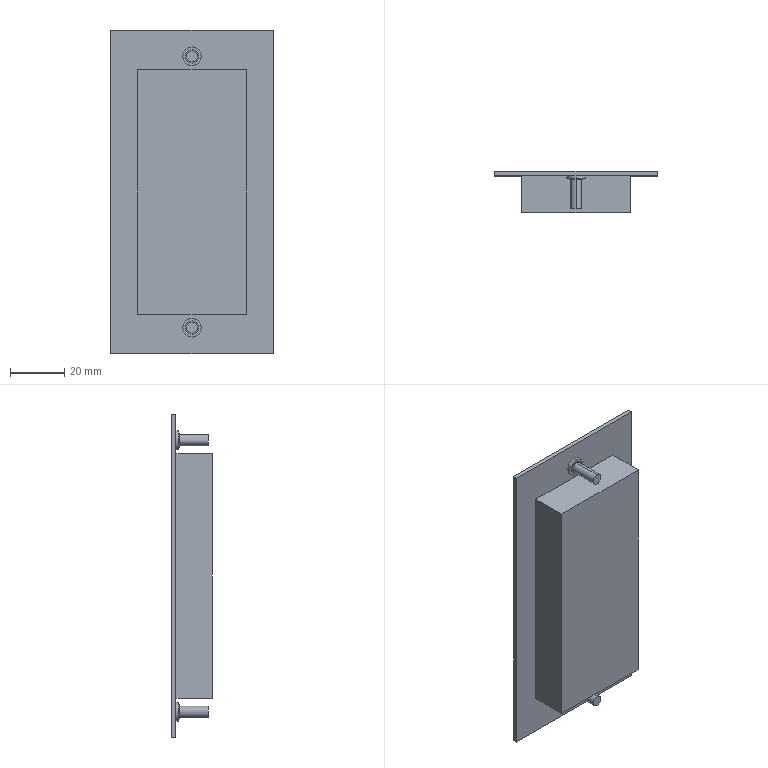Part | STEP file | Concealed handle XAD01_304_Yihe Da | 1 solid | 39 faces | box 60 x 15 x 119 mm | volume 18675 mm3 | plane 27 | cylinder 12 | commonest cylinder face diameters 4 x4 5 x4 6.85 x4